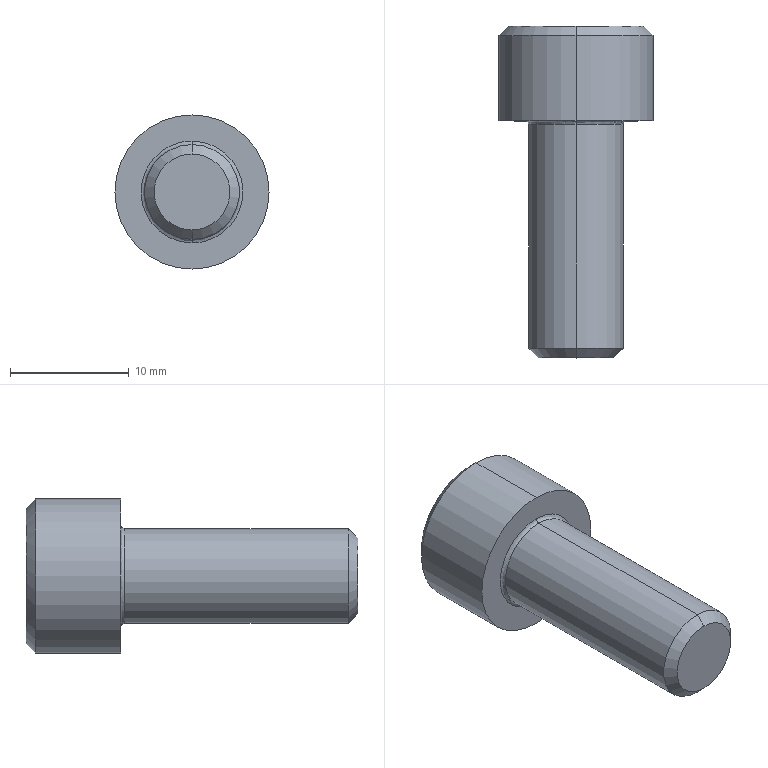Part | STEP file | 1 solid | 20 faces | box 13 x 28 x 13 mm | volume 1861 mm3 | plane 10 | cone 4 | cylinder 4 | spline 2 | commonest cylinder face diameters 8 x2 13 x2